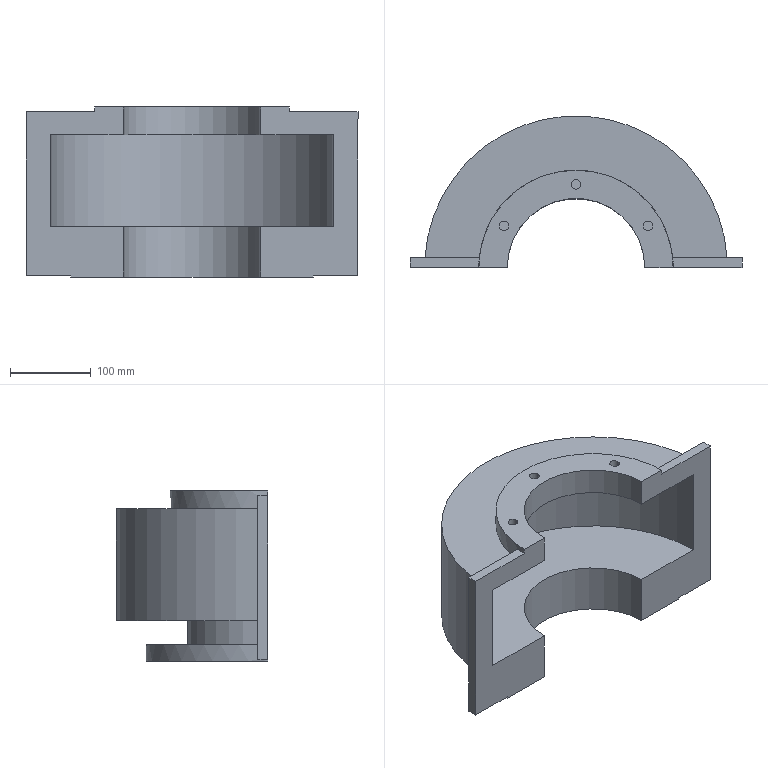Part | SolidWorks | features ICE 6, HoleWzd 2, Extrusion 1, RevCut 1 | 1 solid | 34 faces | box 410 x 187 x 210 mm | volume 2846531 mm3 | cylinder 17 | plane 17 | commonest cylinder face diameters 12 x6 16 x4 170 x2 198 x1 240 x1 300 x1
STEP:
#1=CARTESIAN_POINT('',(515.231,337.244,-184.693));
#2=VERTEX_POINT('',#1);
#3=CARTESIAN_POINT('',(527.231,337.244,-184.693));
#4=VERTEX_POINT('',#3);
#5=CARTESIAN_POINT('',(521.231,337.244,-184.693));
#6=DIRECTION('',(0.,0.,1.));
#7=DIRECTION('',(1.,0.,0.));
#8=AXIS2_PLACEMENT_3D('',#5,#6,#7);
#9=CIRCLE('',#8,6.);
#10=EDGE_CURVE('',#2,#4,#9,.T.);
#11=ORIENTED_EDGE('',*,*,#10,.F.);
#12=CARTESIAN_POINT('',(515.231,337.244,-150.693));
#13=VERTEX_POINT('',#12);
#14=CARTESIAN_POINT('',(515.231,337.244,-150.693));
#15=DIRECTION('',(0.,0.,1.));
#16=VECTOR('',#15,1000.);
#17=LINE('',#14,#16);
#18=EDGE_CURVE('',#2,#13,#17,.T.);
#19=ORIENTED_EDGE('',*,*,#18,.T.);
#20=CARTESIAN_POINT('',(527.231,337.244,-150.693));
#21=VERTEX_POINT('',#20);
#22=CARTESIAN_POINT('',(521.231,337.244,-150.693));
#23=DIRECTION('',(0.,0.,1.));
#24=DIRECTION('',(1.,0.,0.));
#25=AXIS2_PLACEMENT_3D('',#22,#23,#24);
#26=CIRCLE('',#25,6.);
#27=EDGE_CURVE('',#13,#21,#26,.T.);
#28=ORIENTED_EDGE('',*,*,#27,.T.);
#29=CARTESIAN_POINT('',(527.231,337.244,-150.693));
#30=DIRECTION('',(0.,0.,1.));
#31=VECTOR('',#30,1000.);
#32=LINE('',#29,#31);
#33=EDGE_CURVE('',#4,#21,#32,.T.);
#34=ORIENTED_EDGE('',*,*,#33,.F.);
#35=EDGE_LOOP('',(#11,#19,#28,#34));
#36=FACE_OUTER_BOUND('',#35,.T.);
#37=CARTESIAN_POINT('',(521.231,337.244,-150.693));
#38=DIRECTION('',(0.,0.,1.));
#39=DIRECTION('',(1.,0.,0.));
#40=AXIS2_PLACEMENT_3D('',#37,#38,#39);
#41=CYLINDRICAL_SURFACE('',#40,6.);
#42=ADVANCED_FACE('',(#36),#41,.F.);
#43=CARTESIAN_POINT('',(426.463,285.994,-184.693));
#44=VERTEX_POINT('',#43);
#45=CARTESIAN_POINT('',(438.463,285.994,-184.693));
#46=VERTEX_POINT('',#45);
#47=CARTESIAN_POINT('',(432.463,285.994,-184.693));
#48=DIRECTION('',(0.,0.,1.));
#49=DIRECTION('',(1.,0.,0.));
#50=AXIS2_PLACEMENT_3D('',#47,#48,#49);
#51=CIRCLE('',#50,6.);
#52=EDGE_CURVE('',#44,#46,#51,.T.);
#53=ORIENTED_EDGE('',*,*,#52,.F.);
#54=CARTESIAN_POINT('',(426.463,285.994,-150.693));
#55=VERTEX_POINT('',#54);
#56=CARTESIAN_POINT('',(426.463,285.994,-150.693));
#57=DIRECTION('',(0.,0.,1.));
#58=VECTOR('',#57,1000.);
#59=LINE('',#56,#58);
#60=EDGE_CURVE('',#44,#55,#59,.T.);
#61=ORIENTED_EDGE('',*,*,#60,.T.);
#62=CARTESIAN_POINT('',(438.463,285.994,-150.693));
#63=VERTEX_POINT('',#62);
#64=CARTESIAN_POINT('',(432.463,285.994,-150.693));
#65=DIRECTION('',(0.,0.,1.));
#66=DIRECTION('',(1.,0.,0.));
#67=AXIS2_PLACEMENT_3D('',#64,#65,#66);
#68=CIRCLE('',#67,6.);
#69=EDGE_CURVE('',#55,#63,#68,.T.);
#70=ORIENTED_EDGE('',*,*,#69,.T.);
#71=CARTESIAN_POINT('',(438.463,285.994,-150.693));
#72=DIRECTION('',(0.,0.,1.));
#73=VECTOR('',#72,1000.);
#74=LINE('',#71,#73);
#75=EDGE_CURVE('',#46,#63,#74,.T.);
#76=ORIENTED_EDGE('',*,*,#75,.F.);
#77=EDGE_LOOP('',(#53,#61,#70,#76));
#78=FACE_OUTER_BOUND('',#77,.T.);
#79=CARTESIAN_POINT('',(432.463,285.994,-150.693));
#80=DIRECTION('',(0.,0.,1.));
#81=DIRECTION('',(1.,0.,0.));
#82=AXIS2_PLACEMENT_3D('',#79,#80,#81);
#83=CYLINDRICAL_SURFACE('',#82,6.);
#84=ADVANCED_FACE('',(#78),#83,.F.);
#85=CARTESIAN_POINT('',(603.998,285.994,-184.693));
#86=VERTEX_POINT('',#85);
#87=CARTESIAN_POINT('',(615.998,285.994,-184.693));
#88=VERTEX_POINT('',#87);
#89=CARTESIAN_POINT('',(609.998,285.994,-184.693));
#90=DIRECTION('',(0.,0.,1.));
#91=DIRECTION('',(1.,0.,0.));
#92=AXIS2_PLACEMENT_3D('',#89,#90,#91);
#93=CIRCLE('',#92,6.);
#94=EDGE_CURVE('',#86,#88,#93,.T.);
#95=ORIENTED_EDGE('',*,*,#94,.F.);
#96=CARTESIAN_POINT('',(603.998,285.994,-150.693));
#97=VERTEX_POINT('',#96);
#98=CARTESIAN_POINT('',(603.998,285.994,-150.693));
#99=DIRECTION('',(0.,0.,1.));
#100=VECTOR('',#99,1000.);
#101=LINE('',#98,#100);
#102=EDGE_CURVE('',#86,#97,#101,.T.);
#103=ORIENTED_EDGE('',*,*,#102,.T.);
#104=CARTESIAN_POINT('',(615.998,285.994,-150.693));
#105=VERTEX_POINT('',#104);
#106=CARTESIAN_POINT('',(609.998,285.994,-150.693));
#107=DIRECTION('',(0.,0.,1.));
#108=DIRECTION('',(1.,0.,0.));
#109=AXIS2_PLACEMENT_3D('',#106,#107,#108);
#110=CIRCLE('',#109,6.);
#111=EDGE_CURVE('',#97,#105,#110,.T.);
#112=ORIENTED_EDGE('',*,*,#111,.T.);
#113=CARTESIAN_POINT('',(615.998,285.994,-150.693));
#114=DIRECTION('',(0.,0.,1.));
#115=VECTOR('',#114,1000.);
#116=LINE('',#113,#115);
#117=EDGE_CURVE('',#88,#105,#116,.T.);
#118=ORIENTED_EDGE('',*,*,#117,.F.);
#119=EDGE_LOOP('',(#95,#103,#112,#118));
#120=FACE_OUTER_BOUND('',#119,.T.);
#121=CARTESIAN_POINT('',(609.998,285.994,-150.693));
#122=DIRECTION('',(0.,0.,1.));
#123=DIRECTION('',(1.,0.,0.));
#124=AXIS2_PLACEMENT_3D('',#121,#122,#123);
#125=CYLINDRICAL_SURFACE('',#124,6.);
#126=ADVANCED_FACE('',(#120),#125,.F.);
#127=CARTESIAN_POINT('',(413.638,292.244,-360.693));
#128=VERTEX_POINT('',#127);
#129=CARTESIAN_POINT('',(429.638,292.244,-360.693));
#130=VERTEX_POINT('',#129);
#131=CARTESIAN_POINT('',(421.638,292.244,-360.693));
#132=DIRECTION('',(0.,0.,1.));
#133=DIRECTION('',(1.,0.,0.));
#134=AXIS2_PLACEMENT_3D('',#131,#132,#133);
#135=CIRCLE('',#134,8.);
#136=EDGE_CURVE('',#128,#130,#135,.T.);
#137=ORIENTED_EDGE('',*,*,#136,.F.);
#138=CARTESIAN_POINT('',(413.638,292.244,-340.693));
#139=VERTEX_POINT('',#138);
#140=CARTESIAN_POINT('',(413.638,292.244,-340.693));
#141=DIRECTION('',(0.,0.,1.));
#142=VECTOR('',#141,1000.);
#143=LINE('',#140,#142);
#144=EDGE_CURVE('',#128,#139,#143,.T.);
#145=ORIENTED_EDGE('',*,*,#144,.T.);
#146=CARTESIAN_POINT('',(429.638,292.244,-340.693));
#147=VERTEX_POINT('',#146);
#148=CARTESIAN_POINT('',(421.638,292.244,-340.693));
#149=DIRECTION('',(0.,0.,1.));
#150=DIRECTION('',(1.,0.,0.));
#151=AXIS2_PLACEMENT_3D('',#148,#149,#150);
#152=CIRCLE('',#151,8.);
#153=EDGE_CURVE('',#139,#147,#152,.T.);
#154=ORIENTED_EDGE('',*,*,#153,.T.);
#155=CARTESIAN_POINT('',(429.638,292.244,-340.693));
#156=DIRECTION('',(0.,0.,1.));
#157=VECTOR('',#156,1000.);
#158=LINE('',#155,#157);
#159=EDGE_CURVE('',#130,#147,#158,.T.);
#160=ORIENTED_EDGE('',*,*,#159,.F.);
#161=EDGE_LOOP('',(#137,#145,#154,#160));
#162=FACE_OUTER_BOUND('',#161,.T.);
#163=CARTESIAN_POINT('',(421.638,292.244,-340.693));
#164=DIRECTION('',(0.,0.,1.));
#165=DIRECTION('',(1.,0.,0.));
#166=AXIS2_PLACEMENT_3D('',#163,#164,#165);
#167=CYLINDRICAL_SURFACE('',#166,8.);
#168=ADVANCED_FACE('',(#162),#167,.F.);
#169=CARTESIAN_POINT('',(612.824,292.244,-360.693));
#170=VERTEX_POINT('',#169);
#171=CARTESIAN_POINT('',(628.824,292.244,-360.693));
#172=VERTEX_POINT('',#171);
#173=CARTESIAN_POINT('',(620.824,292.244,-360.693));
#174=DIRECTION('',(0.,0.,1.));
#175=DIRECTION('',(1.,0.,0.));
#176=AXIS2_PLACEMENT_3D('',#173,#174,#175);
#177=CIRCLE('',#176,8.);
#178=EDGE_CURVE('',#170,#172,#177,.T.);
#179=ORIENTED_EDGE('',*,*,#178,.F.);
#180=CARTESIAN_POINT('',(612.824,292.244,-340.693));
#181=VERTEX_POINT('',#180);
#182=CARTESIAN_POINT('',(612.824,292.244,-340.693));
#183=DIRECTION('',(0.,0.,1.));
#184=VECTOR('',#183,1000.);
#185=LINE('',#182,#184);
#186=EDGE_CURVE('',#170,#181,#185,.T.);
#187=ORIENTED_EDGE('',*,*,#186,.T.);
#188=CARTESIAN_POINT('',(628.824,292.244,-340.693));
#189=VERTEX_POINT('',#188);
#190=CARTESIAN_POINT('',(620.824,292.244,-340.693));
#191=DIRECTION('',(0.,0.,1.));
#192=DIRECTION('',(1.,0.,0.));
#193=AXIS2_PLACEMENT_3D('',#190,#191,#192);
#194=CIRCLE('',#193,8.);
#195=EDGE_CURVE('',#181,#189,#194,.T.);
#196=ORIENTED_EDGE('',*,*,#195,.T.);
#197=CARTESIAN_POINT('',(628.824,292.244,-340.693));
#198=DIRECTION('',(0.,0.,1.));
#199=VECTOR('',#198,1000.);
#200=LINE('',#197,#199);
#201=EDGE_CURVE('',#172,#189,#200,.T.);
#202=ORIENTED_EDGE('',*,*,#201,.F.);
#203=EDGE_LOOP('',(#179,#187,#196,#202));
#204=FACE_OUTER_BOUND('',#203,.T.);
#205=CARTESIAN_POINT('',(620.824,292.244,-340.693));
#206=DIRECTION('',(0.,0.,1.));
#207=DIRECTION('',(1.,0.,0.));
#208=AXIS2_PLACEMENT_3D('',#205,#206,#207);
#209=CYLINDRICAL_SURFACE('',#208,8.);
#210=ADVANCED_FACE('',(#204),#209,.F.);
#211=CARTESIAN_POINT('',(521.231,337.244,-150.693));
#212=DIRECTION('',(0.,0.,1.));
#213=DIRECTION('',(1.,0.,0.));
#214=AXIS2_PLACEMENT_3D('',#211,#212,#213);
#215=CIRCLE('',#214,6.);
#216=EDGE_CURVE('',#21,#13,#215,.T.);
#217=ORIENTED_EDGE('',*,*,#216,.F.);
#218=ORIENTED_EDGE('',*,*,#27,.F.);
#219=EDGE_LOOP('',(#217,#218));
#220=FACE_BOUND('',#219,.T.);
#221=CARTESIAN_POINT('',(401.231,234.744,-150.693));
#222=VERTEX_POINT('',#221);
#223=CARTESIAN_POINT('',(436.231,234.744,-150.693));
#224=VERTEX_POINT('',#223);
#225=CARTESIAN_POINT('',(641.231,234.744,-150.693));
#226=DIRECTION('',(1.,0.,0.));
#227=VECTOR('',#226,1000.);
#228=LINE('',#225,#227);
#229=EDGE_CURVE('',#222,#224,#228,.T.);
#230=ORIENTED_EDGE('',*,*,#229,.T.);
#231=CARTESIAN_POINT('',(606.231,234.744,-150.693));
#232=VERTEX_POINT('',#231);
#233=CARTESIAN_POINT('',(521.231,234.744,-150.693));
#234=DIRECTION('',(0.,0.,1.));
#235=DIRECTION('',(1.,0.,0.));
#236=AXIS2_PLACEMENT_3D('',#233,#234,#235);
#237=CIRCLE('',#236,85.);
#238=EDGE_CURVE('',#232,#224,#237,.T.);
#239=ORIENTED_EDGE('',*,*,#238,.F.);
#240=CARTESIAN_POINT('',(641.231,234.744,-150.693));
#241=VERTEX_POINT('',#240);
#242=CARTESIAN_POINT('',(641.231,234.744,-150.693));
#243=DIRECTION('',(1.,0.,0.));
#244=VECTOR('',#243,1000.);
#245=LINE('',#242,#244);
#246=EDGE_CURVE('',#232,#241,#245,.T.);
#247=ORIENTED_EDGE('',*,*,#246,.T.);
#248=CARTESIAN_POINT('',(521.231,234.744,-150.693));
#249=DIRECTION('',(0.,0.,1.));
#250=DIRECTION('',(-1.,0.,0.));
#251=AXIS2_PLACEMENT_3D('',#248,#249,#250);
#252=CIRCLE('',#251,120.);
#253=EDGE_CURVE('',#241,#222,#252,.T.);
#254=ORIENTED_EDGE('',*,*,#253,.T.);
#255=EDGE_LOOP('',(#230,#239,#247,#254));
#256=FACE_OUTER_BOUND('',#255,.T.);
#257=CARTESIAN_POINT('',(609.998,285.994,-150.693));
#258=DIRECTION('',(0.,0.,1.));
#259=DIRECTION('',(1.,0.,0.));
#260=AXIS2_PLACEMENT_3D('',#257,#258,#259);
#261=CIRCLE('',#260,6.);
#262=EDGE_CURVE('',#105,#97,#261,.T.);
#263=ORIENTED_EDGE('',*,*,#262,.F.);
#264=ORIENTED_EDGE('',*,*,#111,.F.);
#265=EDGE_LOOP('',(#263,#264));
#266=FACE_BOUND('',#265,.T.);
#267=CARTESIAN_POINT('',(432.463,285.994,-150.693));
#268=DIRECTION('',(0.,0.,1.));
#269=DIRECTION('',(1.,0.,0.));
#270=AXIS2_PLACEMENT_3D('',#267,#268,#269);
#271=CIRCLE('',#270,6.);
#272=EDGE_CURVE('',#63,#55,#271,.T.);
#273=ORIENTED_EDGE('',*,*,#272,.F.);
#274=ORIENTED_EDGE('',*,*,#69,.F.);
#275=EDGE_LOOP('',(#273,#274));
#276=FACE_BOUND('',#275,.T.);
#277=CARTESIAN_POINT('',(521.231,234.744,-150.693));
#278=DIRECTION('',(0.,0.,-1.));
#279=DIRECTION('',(-1.,0.,0.));
#280=AXIS2_PLACEMENT_3D('',#277,#278,#279);
#281=PLANE('',#280);
#282=ADVANCED_FACE('',(#220,#256,#266,#276),#281,.F.);
#283=CARTESIAN_POINT('',(436.231,234.744,-298.693));
#284=VERTEX_POINT('',#283);
#285=CARTESIAN_POINT('',(436.231,234.744,-360.693));
#286=VERTEX_POINT('',#285);
#287=CARTESIAN_POINT('',(436.231,234.744,-360.693));
#288=DIRECTION('',(0.,0.,-1.));
#289=VECTOR('',#288,1000.);
#290=LINE('',#287,#289);
#291=EDGE_CURVE('',#284,#286,#290,.T.);
#292=ORIENTED_EDGE('',*,*,#291,.F.);
#293=CARTESIAN_POINT('',(346.231,234.744,-298.693));
#294=VERTEX_POINT('',#293);
#295=CARTESIAN_POINT('',(726.231,234.744,-298.693));
#296=DIRECTION('',(1.,0.,0.));
#297=VECTOR('',#296,1000.);
#298=LINE('',#295,#297);
#299=EDGE_CURVE('',#294,#284,#298,.T.);
#300=ORIENTED_EDGE('',*,*,#299,.F.);
#301=CARTESIAN_POINT('',(346.231,234.744,-184.693));
#302=VERTEX_POINT('',#301);
#303=CARTESIAN_POINT('',(346.231,234.744,-360.693));
#304=DIRECTION('',(0.,0.,-1.));
#305=VECTOR('',#304,1000.);
#306=LINE('',#303,#305);
#307=EDGE_CURVE('',#302,#294,#306,.T.);
#308=ORIENTED_EDGE('',*,*,#307,.F.);
#309=CARTESIAN_POINT('',(436.231,234.744,-184.693));
#310=VERTEX_POINT('',#309);
#311=CARTESIAN_POINT('',(726.231,234.744,-184.693));
#312=DIRECTION('',(-1.,0.,0.));
#313=VECTOR('',#312,1000.);
#314=LINE('',#311,#313);
#315=EDGE_CURVE('',#310,#302,#314,.T.);
#316=ORIENTED_EDGE('',*,*,#315,.F.);
#317=CARTESIAN_POINT('',(436.231,234.744,-360.693));
#318=DIRECTION('',(0.,0.,-1.));
#319=VECTOR('',#318,1000.);
#320=LINE('',#317,#319);
#321=EDGE_CURVE('',#224,#310,#320,.T.);
#322=ORIENTED_EDGE('',*,*,#321,.F.);
#323=ORIENTED_EDGE('',*,*,#229,.F.);
#324=CARTESIAN_POINT('',(401.231,234.744,-156.693));
#325=VERTEX_POINT('',#324);
#326=CARTESIAN_POINT('',(401.231,234.744,-150.693));
#327=DIRECTION('',(0.,0.,-1.));
#328=VECTOR('',#327,1000.);
#329=LINE('',#326,#328);
#330=EDGE_CURVE('',#222,#325,#329,.T.);
#331=ORIENTED_EDGE('',*,*,#330,.T.);
#332=CARTESIAN_POINT('',(316.231,234.744,-156.693));
#333=VERTEX_POINT('',#332);
#334=CARTESIAN_POINT('',(726.231,234.744,-156.693));
#335=DIRECTION('',(-1.,0.,0.));
#336=VECTOR('',#335,1000.);
#337=LINE('',#334,#336);
#338=EDGE_CURVE('',#325,#333,#337,.T.);
#339=ORIENTED_EDGE('',*,*,#338,.T.);
#340=CARTESIAN_POINT('',(316.231,234.744,-358.693));
#341=VERTEX_POINT('',#340);
#342=CARTESIAN_POINT('',(316.231,234.744,-156.693));
#343=DIRECTION('',(0.,0.,-1.));
#344=VECTOR('',#343,1000.);
#345=LINE('',#342,#344);
#346=EDGE_CURVE('',#333,#341,#345,.T.);
#347=ORIENTED_EDGE('',*,*,#346,.T.);
#348=CARTESIAN_POINT('',(371.231,234.744,-358.693));
#349=VERTEX_POINT('',#348);
#350=CARTESIAN_POINT('',(726.231,234.744,-358.693));
#351=DIRECTION('',(-1.,0.,0.));
#352=VECTOR('',#351,1000.);
#353=LINE('',#350,#352);
#354=EDGE_CURVE('',#349,#341,#353,.T.);
#355=ORIENTED_EDGE('',*,*,#354,.F.);
#356=CARTESIAN_POINT('',(371.231,234.744,-360.693));
#357=VERTEX_POINT('',#356);
#358=CARTESIAN_POINT('',(371.231,234.744,-360.693));
#359=DIRECTION('',(0.,0.,1.));
#360=VECTOR('',#359,1000.);
#361=LINE('',#358,#360);
#362=EDGE_CURVE('',#357,#349,#361,.T.);
#363=ORIENTED_EDGE('',*,*,#362,.F.);
#364=CARTESIAN_POINT('',(371.231,234.744,-360.693));
#365=DIRECTION('',(-1.,0.,0.));
#366=VECTOR('',#365,1000.);
#367=LINE('',#364,#366);
#368=EDGE_CURVE('',#286,#357,#367,.T.);
#369=ORIENTED_EDGE('',*,*,#368,.F.);
#370=EDGE_LOOP('',(#292,#300,#308,#316,#322,#323,#331,#339,#347,#355,#363,#369));
#371=FACE_OUTER_BOUND('',#370,.T.);
#372=CARTESIAN_POINT('',(726.231,234.744,-156.693));
#373=DIRECTION('',(0.,-1.,0.));
#374=DIRECTION('',(1.,0.,0.));
#375=AXIS2_PLACEMENT_3D('',#372,#373,#374);
#376=PLANE('',#375);
#377=ADVANCED_FACE('',(#371),#376,.T.);
#378=CARTESIAN_POINT('',(670.75,246.744,-340.693));
#379=VERTEX_POINT('',#378);
#380=CARTESIAN_POINT('',(619.501,246.744,-340.693));
#381=VERTEX_POINT('',#380);
#382=CARTESIAN_POINT('',(707.845,246.744,-340.693));
#383=DIRECTION('',(-1.,0.,0.));
#384=VECTOR('',#383,1000.);
#385=LINE('',#382,#384);
#386=EDGE_CURVE('',#379,#381,#385,.T.);
#387=ORIENTED_EDGE('',*,*,#386,.T.);
#388=CARTESIAN_POINT('',(619.501,246.744,-310.693));
#389=VERTEX_POINT('',#388);
#390=CARTESIAN_POINT('',(619.501,246.744,-310.693));
#391=DIRECTION('',(0.,0.,-1.));
#392=VECTOR('',#391,1000.);
#393=LINE('',#390,#392);
#394=EDGE_CURVE('',#389,#381,#393,.T.);
#395=ORIENTED_EDGE('',*,*,#394,.F.);
#396=CARTESIAN_POINT('',(707.845,246.744,-310.693));
#397=VERTEX_POINT('',#396);
#398=CARTESIAN_POINT('',(707.845,246.744,-310.693));
#399=DIRECTION('',(-1.,0.,0.));
#400=VECTOR('',#399,1000.);
#401=LINE('',#398,#400);
#402=EDGE_CURVE('',#397,#389,#401,.T.);
#403=ORIENTED_EDGE('',*,*,#402,.F.);
#404=CARTESIAN_POINT('',(707.845,246.744,-172.693));
#405=VERTEX_POINT('',#404);
#406=CARTESIAN_POINT('',(707.845,246.744,-156.693));
#407=DIRECTION('',(0.,0.,-1.));
#408=VECTOR('',#407,1000.);
#409=LINE('',#406,#408);
#410=EDGE_CURVE('',#405,#397,#409,.T.);
#411=ORIENTED_EDGE('',*,*,#410,.F.);
#412=CARTESIAN_POINT('',(640.629,246.744,-172.693));
#413=VERTEX_POINT('',#412);
#414=CARTESIAN_POINT('',(640.629,246.744,-172.693));
#415=DIRECTION('',(1.,0.,0.));
#416=VECTOR('',#415,1000.);
#417=LINE('',#414,#416);
#418=EDGE_CURVE('',#413,#405,#417,.T.);
#419=ORIENTED_EDGE('',*,*,#418,.F.);
#420=CARTESIAN_POINT('',(640.629,246.744,-156.693));
#421=VERTEX_POINT('',#420);
#422=CARTESIAN_POINT('',(640.629,246.744,-172.693));
#423=DIRECTION('',(0.,0.,1.));
#424=VECTOR('',#423,1000.);
#425=LINE('',#422,#424);
#426=EDGE_CURVE('',#413,#421,#425,.T.);
#427=ORIENTED_EDGE('',*,*,#426,.T.);
#428=CARTESIAN_POINT('',(726.231,246.744,-156.693));
#429=VERTEX_POINT('',#428);
#430=CARTESIAN_POINT('',(707.845,246.744,-156.693));
#431=DIRECTION('',(1.,0.,0.));
#432=VECTOR('',#431,1000.);
#433=LINE('',#430,#432);
#434=EDGE_CURVE('',#421,#429,#433,.T.);
#435=ORIENTED_EDGE('',*,*,#434,.T.);
#436=CARTESIAN_POINT('',(726.231,246.744,-358.693));
#437=VERTEX_POINT('',#436);
#438=CARTESIAN_POINT('',(726.231,246.744,-156.693));
#439=DIRECTION('',(0.,0.,-1.));
#440=VECTOR('',#439,1000.);
#441=LINE('',#438,#440);
#442=EDGE_CURVE('',#429,#437,#441,.T.);
#443=ORIENTED_EDGE('',*,*,#442,.T.);
#444=CARTESIAN_POINT('',(670.75,246.744,-358.693));
#445=VERTEX_POINT('',#444);
#446=CARTESIAN_POINT('',(707.845,246.744,-358.693));
#447=DIRECTION('',(1.,0.,0.));
#448=VECTOR('',#447,1000.);
#449=LINE('',#446,#448);
#450=EDGE_CURVE('',#445,#437,#449,.T.);
#451=ORIENTED_EDGE('',*,*,#450,.F.);
#452=CARTESIAN_POINT('',(670.75,246.744,-340.693));
#453=DIRECTION('',(0.,0.,-1.));
#454=VECTOR('',#453,1000.);
#455=LINE('',#452,#454);
#456=EDGE_CURVE('',#379,#445,#455,.T.);
#457=ORIENTED_EDGE('',*,*,#456,.F.);
#458=EDGE_LOOP('',(#387,#395,#403,#411,#419,#427,#435,#443,#451,#457));
#459=FACE_OUTER_BOUND('',#458,.T.);
#460=CARTESIAN_POINT('',(316.231,246.744,-156.693));
#461=DIRECTION('',(0.,1.,0.));
#462=DIRECTION('',(0.,0.,1.));
#463=AXIS2_PLACEMENT_3D('',#460,#461,#462);
#464=PLANE('',#463);
#465=ADVANCED_FACE('',(#459),#464,.T.);
#466=CARTESIAN_POINT('',(422.961,246.744,-310.693));
#467=VERTEX_POINT('',#466);
#468=CARTESIAN_POINT('',(334.616,246.744,-310.693));
#469=VERTEX_POINT('',#468);
#470=CARTESIAN_POINT('',(707.845,246.744,-310.693));
#471=DIRECTION('',(-1.,0.,0.));
#472=VECTOR('',#471,1000.);
#473=LINE('',#470,#472);
#474=EDGE_CURVE('',#467,#469,#473,.T.);
#475=ORIENTED_EDGE('',*,*,#474,.F.);
#476=CARTESIAN_POINT('',(422.961,246.744,-340.693));
#477=VERTEX_POINT('',#476);
#478=CARTESIAN_POINT('',(422.961,246.744,-310.693));
#479=DIRECTION('',(0.,0.,-1.));
#480=VECTOR('',#479,1000.);
#481=LINE('',#478,#480);
#482=EDGE_CURVE('',#467,#477,#481,.T.);
#483=ORIENTED_EDGE('',*,*,#482,.T.);
#484=CARTESIAN_POINT('',(371.711,246.744,-340.693));
#485=VERTEX_POINT('',#484);
#486=CARTESIAN_POINT('',(707.845,246.744,-340.693));
#487=DIRECTION('',(-1.,0.,0.));
#488=VECTOR('',#487,1000.);
#489=LINE('',#486,#488);
#490=EDGE_CURVE('',#477,#485,#489,.T.);
#491=ORIENTED_EDGE('',*,*,#490,.T.);
#492=CARTESIAN_POINT('',(371.711,246.744,-358.693));
#493=VERTEX_POINT('',#492);
#494=CARTESIAN_POINT('',(371.711,246.744,-340.693));
#495=DIRECTION('',(0.,0.,-1.));
#496=VECTOR('',#495,1000.);
#497=LINE('',#494,#496);
#498=EDGE_CURVE('',#485,#493,#497,.T.);
#499=ORIENTED_EDGE('',*,*,#498,.T.);
#500=CARTESIAN_POINT('',(316.231,246.744,-358.693));
#501=VERTEX_POINT('',#500);
#502=CARTESIAN_POINT('',(316.231,246.744,-358.693));
#503=DIRECTION('',(1.,0.,0.));
#504=VECTOR('',#503,1000.);
#505=LINE('',#502,#504);
#506=EDGE_CURVE('',#501,#493,#505,.T.);
#507=ORIENTED_EDGE('',*,*,#506,.F.);
#508=CARTESIAN_POINT('',(316.231,246.744,-156.693));
#509=VERTEX_POINT('',#508);
#510=CARTESIAN_POINT('',(316.231,246.744,-156.693));
#511=DIRECTION('',(0.,0.,-1.));
#512=VECTOR('',#511,1000.);
#513=LINE('',#510,#512);
#514=EDGE_CURVE('',#509,#501,#513,.T.);
#515=ORIENTED_EDGE('',*,*,#514,.F.);
#516=CARTESIAN_POINT('',(401.832,246.744,-156.693));
#517=VERTEX_POINT('',#516);
#518=CARTESIAN_POINT('',(316.231,246.744,-156.693));
#519=DIRECTION('',(1.,0.,0.));
#520=VECTOR('',#519,1000.);
#521=LINE('',#518,#520);
#522=EDGE_CURVE('',#509,#517,#521,.T.);
#523=ORIENTED_EDGE('',*,*,#522,.T.);
#524=CARTESIAN_POINT('',(401.832,246.744,-172.693));
#525=VERTEX_POINT('',#524);
#526=CARTESIAN_POINT('',(401.832,246.744,-172.693));
#527=DIRECTION('',(0.,0.,1.));
#528=VECTOR('',#527,1000.);
#529=LINE('',#526,#528);
#530=EDGE_CURVE('',#525,#517,#529,.T.);
#531=ORIENTED_EDGE('',*,*,#530,.F.);
#532=CARTESIAN_POINT('',(334.616,246.744,-172.693));
#533=VERTEX_POINT('',#532);
#534=CARTESIAN_POINT('',(334.616,246.744,-172.693));
#535=DIRECTION('',(1.,0.,0.));
#536=VECTOR('',#535,1000.);
#537=LINE('',#534,#536);
#538=EDGE_CURVE('',#533,#525,#537,.T.);
#539=ORIENTED_EDGE('',*,*,#538,.F.);
#540=CARTESIAN_POINT('',(334.616,246.744,-156.693));
#541=DIRECTION('',(0.,0.,-1.));
#542=VECTOR('',#541,1000.);
#543=LINE('',#540,#542);
#544=EDGE_CURVE('',#533,#469,#543,.T.);
#545=ORIENTED_EDGE('',*,*,#544,.T.);
#546=EDGE_LOOP('',(#475,#483,#491,#499,#507,#515,#523,#531,#539,#545));
#547=FACE_OUTER_BOUND('',#546,.T.);
#548=CARTESIAN_POINT('',(316.231,246.744,-156.693));
#549=DIRECTION('',(0.,1.,0.));
#550=DIRECTION('',(0.,0.,1.));
#551=AXIS2_PLACEMENT_3D('',#548,#549,#550);
#552=PLANE('',#551);
#553=ADVANCED_FACE('',(#547),#552,.T.);
#554=CARTESIAN_POINT('',(421.638,292.244,-340.693));
#555=DIRECTION('',(0.,0.,1.));
#556=DIRECTION('',(1.,0.,0.));
#557=AXIS2_PLACEMENT_3D('',#554,#555,#556);
#558=CIRCLE('',#557,8.);
#559=EDGE_CURVE('',#147,#139,#558,.T.);
#560=ORIENTED_EDGE('',*,*,#559,.F.);
#561=ORIENTED_EDGE('',*,*,#153,.F.);
#562=EDGE_LOOP('',(#560,#561));
#563=FACE_BOUND('',#562,.T.);
#564=CARTESIAN_POINT('',(620.824,292.244,-340.693));
#565=DIRECTION('',(0.,0.,1.));
#566=DIRECTION('',(1.,0.,0.));
#567=AXIS2_PLACEMENT_3D('',#564,#565,#566);
#568=CIRCLE('',#567,8.);
#569=EDGE_CURVE('',#189,#181,#568,.T.);
#570=ORIENTED_EDGE('',*,*,#569,.F.);
#571=ORIENTED_EDGE('',*,*,#195,.F.);
#572=EDGE_LOOP('',(#570,#571));
#573=FACE_BOUND('',#572,.T.);
#574=CARTESIAN_POINT('',(521.231,234.744,-340.693));
#575=DIRECTION('',(0.,0.,1.));
#576=DIRECTION('',(-1.,0.,0.));
#577=AXIS2_PLACEMENT_3D('',#574,#575,#576);
#578=CIRCLE('',#577,99.);
#579=EDGE_CURVE('',#381,#477,#578,.T.);
#580=ORIENTED_EDGE('',*,*,#579,.F.);
#581=ORIENTED_EDGE('',*,*,#386,.F.);
#582=CARTESIAN_POINT('',(521.231,234.744,-340.693));
#583=DIRECTION('',(0.,0.,1.));
#584=DIRECTION('',(1.,0.,0.));
#585=AXIS2_PLACEMENT_3D('',#582,#583,#584);
#586=CIRCLE('',#585,150.);
#587=EDGE_CURVE('',#379,#485,#586,.T.);
#588=ORIENTED_EDGE('',*,*,#587,.T.);
#589=ORIENTED_EDGE('',*,*,#490,.F.);
#590=EDGE_LOOP('',(#580,#581,#588,#589));
#591=FACE_OUTER_BOUND('',#590,.T.);
#592=CARTESIAN_POINT('',(521.231,234.744,-340.693));
#593=DIRECTION('',(0.,0.,-1.));
#594=DIRECTION('',(-1.,0.,0.));
#595=AXIS2_PLACEMENT_3D('',#592,#593,#594);
#596=PLANE('',#595);
#597=ADVANCED_FACE('',(#563,#573,#591),#596,.F.);
#598=ORIENTED_EDGE('',*,*,#402,.T.);
#599=CARTESIAN_POINT('',(521.231,234.744,-310.693));
#600=DIRECTION('',(0.,0.,1.));
#601=DIRECTION('',(-1.,0.,0.));
#602=AXIS2_PLACEMENT_3D('',#599,#600,#601);
#603=CIRCLE('',#602,99.);
#604=EDGE_CURVE('',#389,#467,#603,.T.);
#605=ORIENTED_EDGE('',*,*,#604,.T.);
#606=ORIENTED_EDGE('',*,*,#474,.T.);
#607=CARTESIAN_POINT('',(521.231,234.744,-310.693));
#608=DIRECTION('',(0.,0.,-1.));
#609=DIRECTION('',(-1.,0.,0.));
#610=AXIS2_PLACEMENT_3D('',#607,#608,#609);
#611=CIRCLE('',#610,187.);
#612=EDGE_CURVE('',#469,#397,#611,.T.);
#613=ORIENTED_EDGE('',*,*,#612,.T.);
#614=EDGE_LOOP('',(#598,#605,#606,#613));
#615=FACE_OUTER_BOUND('',#614,.T.);
#616=CARTESIAN_POINT('',(521.231,234.744,-310.693));
#617=DIRECTION('',(0.,0.,-1.));
#618=DIRECTION('',(-1.,0.,0.));
#619=AXIS2_PLACEMENT_3D('',#616,#617,#618);
#620=PLANE('',#619);
#621=ADVANCED_FACE('',(#615),#620,.T.);
#622=CARTESIAN_POINT('',(641.231,234.744,-156.693));
#623=VERTEX_POINT('',#622);
#624=CARTESIAN_POINT('',(521.231,234.744,-156.693));
#625=DIRECTION('',(0.,0.,1.));
#626=DIRECTION('',(-1.,0.,0.));
#627=AXIS2_PLACEMENT_3D('',#624,#625,#626);
#628=CIRCLE('',#627,120.);
#629=EDGE_CURVE('',#623,#421,#628,.T.);
#630=ORIENTED_EDGE('',*,*,#629,.F.);
#631=CARTESIAN_POINT('',(726.231,234.744,-156.693));
#632=VERTEX_POINT('',#631);
#633=CARTESIAN_POINT('',(726.231,234.744,-156.693));
#634=DIRECTION('',(-1.,0.,0.));
#635=VECTOR('',#634,1000.);
#636=LINE('',#633,#635);
#637=EDGE_CURVE('',#632,#623,#636,.T.);
#638=ORIENTED_EDGE('',*,*,#637,.F.);
#639=CARTESIAN_POINT('',(726.231,246.744,-156.693));
#640=DIRECTION('',(0.,-1.,0.));
#641=VECTOR('',#640,1000.);
#642=LINE('',#639,#641);
#643=EDGE_CURVE('',#429,#632,#642,.T.);
#644=ORIENTED_EDGE('',*,*,#643,.F.);
#645=ORIENTED_EDGE('',*,*,#434,.F.);
#646=EDGE_LOOP('',(#630,#638,#644,#645));
#647=FACE_OUTER_BOUND('',#646,.T.);
#648=CARTESIAN_POINT('',(521.231,234.744,-156.693));
#649=DIRECTION('',(0.,0.,-1.));
#650=DIRECTION('',(-1.,0.,0.));
#651=AXIS2_PLACEMENT_3D('',#648,#649,#650);
#652=PLANE('',#651);
#653=ADVANCED_FACE('',(#647),#652,.F.);
#654=CARTESIAN_POINT('',(521.231,234.744,-358.693));
#655=DIRECTION('',(0.,0.,-1.));
#656=DIRECTION('',(1.,0.,0.));
#657=AXIS2_PLACEMENT_3D('',#654,#655,#656);
#658=CIRCLE('',#657,150.);
#659=EDGE_CURVE('',#349,#493,#658,.T.);
#660=ORIENTED_EDGE('',*,*,#659,.F.);
#661=ORIENTED_EDGE('',*,*,#354,.T.);
#662=CARTESIAN_POINT('',(316.231,234.744,-358.693));
#663=DIRECTION('',(0.,1.,0.));
#664=VECTOR('',#663,1000.);
#665=LINE('',#662,#664);
#666=EDGE_CURVE('',#341,#501,#665,.T.);
#667=ORIENTED_EDGE('',*,*,#666,.T.);
#668=ORIENTED_EDGE('',*,*,#506,.T.);
#669=EDGE_LOOP('',(#660,#661,#667,#668));
#670=FACE_OUTER_BOUND('',#669,.T.);
#671=CARTESIAN_POINT('',(521.231,234.744,-358.693));
#672=DIRECTION('',(0.,0.,-1.));
#673=DIRECTION('',(-1.,0.,0.));
#674=AXIS2_PLACEMENT_3D('',#671,#672,#673);
#675=PLANE('',#674);
#676=ADVANCED_FACE('',(#670),#675,.T.);
#677=ORIENTED_EDGE('',*,*,#410,.T.);
#678=ORIENTED_EDGE('',*,*,#612,.F.);
#679=ORIENTED_EDGE('',*,*,#544,.F.);
#680=CARTESIAN_POINT('',(521.231,234.744,-172.693));
#681=DIRECTION('',(0.,0.,1.));
#682=DIRECTION('',(1.,0.,0.));
#683=AXIS2_PLACEMENT_3D('',#680,#681,#682);
#684=CIRCLE('',#683,187.);
#685=EDGE_CURVE('',#405,#533,#684,.T.);
#686=ORIENTED_EDGE('',*,*,#685,.F.);
#687=EDGE_LOOP('',(#677,#678,#679,#686));
#688=FACE_OUTER_BOUND('',#687,.T.);
#689=CARTESIAN_POINT('',(521.231,234.744,-156.693));
#690=DIRECTION('',(0.,0.,-1.));
#691=DIRECTION('',(-1.,0.,0.));
#692=AXIS2_PLACEMENT_3D('',#689,#690,#691);
#693=CYLINDRICAL_SURFACE('',#692,187.);
#694=ADVANCED_FACE('',(#688),#693,.T.);
#695=ORIENTED_EDGE('',*,*,#666,.F.);
#696=ORIENTED_EDGE('',*,*,#346,.F.);
#697=CARTESIAN_POINT('',(316.231,234.744,-156.693));
#698=DIRECTION('',(0.,1.,0.));
#699=VECTOR('',#698,1000.);
#700=LINE('',#697,#699);
#701=EDGE_CURVE('',#333,#509,#700,.T.);
#702=ORIENTED_EDGE('',*,*,#701,.T.);
#703=ORIENTED_EDGE('',*,*,#514,.T.);
#704=EDGE_LOOP('',(#695,#696,#702,#703));
#705=FACE_OUTER_BOUND('',#704,.T.);
#706=CARTESIAN_POINT('',(316.231,234.744,-156.693));
#707=DIRECTION('',(-1.,0.,0.));
#708=DIRECTION('',(0.,0.,1.));
#709=AXIS2_PLACEMENT_3D('',#706,#707,#708);
#710=PLANE('',#709);
#711=ADVANCED_FACE('',(#705),#710,.T.);
#712=CARTESIAN_POINT('',(606.231,234.744,-360.693));
#713=VERTEX_POINT('',#712);
#714=CARTESIAN_POINT('',(606.231,234.744,-298.693));
#715=VERTEX_POINT('',#714);
#716=CARTESIAN_POINT('',(606.231,234.744,-360.693));
#717=DIRECTION('',(0.,0.,1.));
#718=VECTOR('',#717,1000.);
#719=LINE('',#716,#718);
#720=EDGE_CURVE('',#713,#715,#719,.T.);
#721=ORIENTED_EDGE('',*,*,#720,.F.);
#722=CARTESIAN_POINT('',(671.231,234.744,-360.693));
#723=VERTEX_POINT('',#722);
#724=CARTESIAN_POINT('',(371.231,234.744,-360.693));
#725=DIRECTION('',(-1.,0.,0.));
#726=VECTOR('',#725,1000.);
#727=LINE('',#724,#726);
#728=EDGE_CURVE('',#723,#713,#727,.T.);
#729=ORIENTED_EDGE('',*,*,#728,.F.);
#730=CARTESIAN_POINT('',(671.231,234.744,-358.693));
#731=VERTEX_POINT('',#730);
#732=CARTESIAN_POINT('',(671.231,234.744,-360.693));
#733=DIRECTION('',(0.,0.,1.));
#734=VECTOR('',#733,1000.);
#735=LINE('',#732,#734);
#736=EDGE_CURVE('',#723,#731,#735,.T.);
#737=ORIENTED_EDGE('',*,*,#736,.T.);
#738=CARTESIAN_POINT('',(726.231,234.744,-358.693));
#739=VERTEX_POINT('',#738);
#740=CARTESIAN_POINT('',(726.231,234.744,-358.693));
#741=DIRECTION('',(-1.,0.,0.));
#742=VECTOR('',#741,1000.);
#743=LINE('',#740,#742);
#744=EDGE_CURVE('',#739,#731,#743,.T.);
#745=ORIENTED_EDGE('',*,*,#744,.F.);
#746=CARTESIAN_POINT('',(726.231,234.744,-156.693));
#747=DIRECTION('',(0.,0.,-1.));
#748=VECTOR('',#747,1000.);
#749=LINE('',#746,#748);
#750=EDGE_CURVE('',#632,#739,#749,.T.);
#751=ORIENTED_EDGE('',*,*,#750,.F.);
#752=ORIENTED_EDGE('',*,*,#637,.T.);
#753=CARTESIAN_POINT('',(641.231,234.744,-150.693));
#754=DIRECTION('',(0.,0.,-1.));
#755=VECTOR('',#754,1000.);
#756=LINE('',#753,#755);
#757=EDGE_CURVE('',#241,#623,#756,.T.);
#758=ORIENTED_EDGE('',*,*,#757,.F.);
#759=ORIENTED_EDGE('',*,*,#246,.F.);
#760=CARTESIAN_POINT('',(606.231,234.744,-184.693));
#761=VERTEX_POINT('',#760);
#762=CARTESIAN_POINT('',(606.231,234.744,-360.693));
#763=DIRECTION('',(0.,0.,1.));
#764=VECTOR('',#763,1000.);
#765=LINE('',#762,#764);
#766=EDGE_CURVE('',#761,#232,#765,.T.);
#767=ORIENTED_EDGE('',*,*,#766,.F.);
#768=CARTESIAN_POINT('',(696.231,234.744,-184.693));
#769=VERTEX_POINT('',#768);
#770=CARTESIAN_POINT('',(726.231,234.744,-184.693));
#771=DIRECTION('',(-1.,0.,0.));
#772=VECTOR('',#771,1000.);
#773=LINE('',#770,#772);
#774=EDGE_CURVE('',#769,#761,#773,.T.);
#775=ORIENTED_EDGE('',*,*,#774,.F.);
#776=CARTESIAN_POINT('',(696.231,234.744,-298.693));
#777=VERTEX_POINT('',#776);
#778=CARTESIAN_POINT('',(696.231,234.744,-360.693));
#779=DIRECTION('',(0.,0.,1.));
#780=VECTOR('',#779,1000.);
#781=LINE('',#778,#780);
#782=EDGE_CURVE('',#777,#769,#781,.T.);
#783=ORIENTED_EDGE('',*,*,#782,.F.);
#784=CARTESIAN_POINT('',(726.231,234.744,-298.693));
#785=DIRECTION('',(1.,0.,0.));
#786=VECTOR('',#785,1000.);
#787=LINE('',#784,#786);
#788=EDGE_CURVE('',#715,#777,#787,.T.);
#789=ORIENTED_EDGE('',*,*,#788,.F.);
#790=EDGE_LOOP('',(#721,#729,#737,#745,#751,#752,#758,#759,#767,#775,#783,#789));
#791=FACE_OUTER_BOUND('',#790,.T.);
#792=CARTESIAN_POINT('',(726.231,234.744,-156.693));
#793=DIRECTION('',(0.,-1.,0.));
#794=DIRECTION('',(1.,0.,0.));
#795=AXIS2_PLACEMENT_3D('',#792,#793,#794);
#796=PLANE('',#795);
#797=ADVANCED_FACE('',(#791),#796,.T.);
#798=CARTESIAN_POINT('',(726.231,246.744,-358.693));
#799=DIRECTION('',(0.,-1.,0.));
#800=VECTOR('',#799,1000.);
#801=LINE('',#798,#800);
#802=EDGE_CURVE('',#437,#739,#801,.T.);
#803=ORIENTED_EDGE('',*,*,#802,.F.);
#804=ORIENTED_EDGE('',*,*,#442,.F.);
#805=ORIENTED_EDGE('',*,*,#643,.T.);
#806=ORIENTED_EDGE('',*,*,#750,.T.);
#807=EDGE_LOOP('',(#803,#804,#805,#806));
#808=FACE_OUTER_BOUND('',#807,.T.);
#809=CARTESIAN_POINT('',(726.231,246.744,-156.693));
#810=DIRECTION('',(1.,0.,0.));
#811=DIRECTION('',(0.,0.,-1.));
#812=AXIS2_PLACEMENT_3D('',#809,#810,#811);
#813=PLANE('',#812);
#814=ADVANCED_FACE('',(#808),#813,.T.);
#815=CARTESIAN_POINT('',(521.231,234.744,-156.693));
#816=DIRECTION('',(0.,0.,1.));
#817=DIRECTION('',(-1.,0.,0.));
#818=AXIS2_PLACEMENT_3D('',#815,#816,#817);
#819=CIRCLE('',#818,120.);
#820=EDGE_CURVE('',#517,#325,#819,.T.);
#821=ORIENTED_EDGE('',*,*,#820,.F.);
#822=ORIENTED_EDGE('',*,*,#522,.F.);
#823=ORIENTED_EDGE('',*,*,#701,.F.);
#824=ORIENTED_EDGE('',*,*,#338,.F.);
#825=EDGE_LOOP('',(#821,#822,#823,#824));
#826=FACE_OUTER_BOUND('',#825,.T.);
#827=CARTESIAN_POINT('',(521.231,234.744,-156.693));
#828=DIRECTION('',(0.,0.,-1.));
#829=DIRECTION('',(-1.,0.,0.));
#830=AXIS2_PLACEMENT_3D('',#827,#828,#829);
#831=PLANE('',#830);
#832=ADVANCED_FACE('',(#826),#831,.F.);
#833=CARTESIAN_POINT('',(521.231,234.744,-358.693));
#834=DIRECTION('',(0.,0.,-1.));
#835=DIRECTION('',(1.,0.,0.));
#836=AXIS2_PLACEMENT_3D('',#833,#834,#835);
#837=CIRCLE('',#836,150.);
#838=EDGE_CURVE('',#445,#731,#837,.T.);
#839=ORIENTED_EDGE('',*,*,#838,.F.);
#840=ORIENTED_EDGE('',*,*,#450,.T.);
#841=ORIENTED_EDGE('',*,*,#802,.T.);
#842=ORIENTED_EDGE('',*,*,#744,.T.);
#843=EDGE_LOOP('',(#839,#840,#841,#842));
#844=FACE_OUTER_BOUND('',#843,.T.);
#845=CARTESIAN_POINT('',(521.231,234.744,-358.693));
#846=DIRECTION('',(0.,0.,-1.));
#847=DIRECTION('',(-1.,0.,0.));
#848=AXIS2_PLACEMENT_3D('',#845,#846,#847);
#849=PLANE('',#848);
#850=ADVANCED_FACE('',(#844),#849,.T.);
#851=ORIENTED_EDGE('',*,*,#530,.T.);
#852=ORIENTED_EDGE('',*,*,#820,.T.);
#853=ORIENTED_EDGE('',*,*,#330,.F.);
#854=ORIENTED_EDGE('',*,*,#253,.F.);
#855=ORIENTED_EDGE('',*,*,#757,.T.);
#856=ORIENTED_EDGE('',*,*,#629,.T.);
#857=ORIENTED_EDGE('',*,*,#426,.F.);
#858=CARTESIAN_POINT('',(521.231,234.744,-172.693));
#859=DIRECTION('',(0.,0.,-1.));
#860=DIRECTION('',(-1.,0.,0.));
#861=AXIS2_PLACEMENT_3D('',#858,#859,#860);
#862=CIRCLE('',#861,120.);
#863=EDGE_CURVE('',#525,#413,#862,.T.);
#864=ORIENTED_EDGE('',*,*,#863,.F.);
#865=EDGE_LOOP('',(#851,#852,#853,#854,#855,#856,#857,#864));
#866=FACE_OUTER_BOUND('',#865,.T.);
#867=CARTESIAN_POINT('',(521.231,234.744,-172.693));
#868=DIRECTION('',(0.,0.,1.));
#869=DIRECTION('',(1.,0.,0.));
#870=AXIS2_PLACEMENT_3D('',#867,#868,#869);
#871=CYLINDRICAL_SURFACE('',#870,120.);
#872=ADVANCED_FACE('',(#866),#871,.T.);
#873=ORIENTED_EDGE('',*,*,#863,.T.);
#874=ORIENTED_EDGE('',*,*,#418,.T.);
#875=ORIENTED_EDGE('',*,*,#685,.T.);
#876=ORIENTED_EDGE('',*,*,#538,.T.);
#877=EDGE_LOOP('',(#873,#874,#875,#876));
#878=FACE_OUTER_BOUND('',#877,.T.);
#879=CARTESIAN_POINT('',(521.231,234.744,-172.693));
#880=DIRECTION('',(0.,0.,-1.));
#881=DIRECTION('',(-1.,0.,0.));
#882=AXIS2_PLACEMENT_3D('',#879,#880,#881);
#883=PLANE('',#882);
#884=ADVANCED_FACE('',(#878),#883,.F.);
#885=ORIENTED_EDGE('',*,*,#456,.T.);
#886=ORIENTED_EDGE('',*,*,#838,.T.);
#887=ORIENTED_EDGE('',*,*,#736,.F.);
#888=CARTESIAN_POINT('',(521.231,234.744,-360.693));
#889=DIRECTION('',(0.,0.,-1.));
#890=DIRECTION('',(1.,0.,0.));
#891=AXIS2_PLACEMENT_3D('',#888,#889,#890);
#892=CIRCLE('',#891,150.);
#893=EDGE_CURVE('',#357,#723,#892,.T.);
#894=ORIENTED_EDGE('',*,*,#893,.F.);
#895=ORIENTED_EDGE('',*,*,#362,.T.);
#896=ORIENTED_EDGE('',*,*,#659,.T.);
#897=ORIENTED_EDGE('',*,*,#498,.F.);
#898=ORIENTED_EDGE('',*,*,#587,.F.);
#899=EDGE_LOOP('',(#885,#886,#887,#894,#895,#896,#897,#898));
#900=FACE_OUTER_BOUND('',#899,.T.);
#901=CARTESIAN_POINT('',(521.231,234.744,-340.693));
#902=DIRECTION('',(0.,0.,-1.));
#903=DIRECTION('',(-1.,0.,0.));
#904=AXIS2_PLACEMENT_3D('',#901,#902,#903);
#905=CYLINDRICAL_SURFACE('',#904,150.);
#906=ADVANCED_FACE('',(#900),#905,.T.);
#907=CARTESIAN_POINT('',(421.638,292.244,-360.693));
#908=DIRECTION('',(0.,0.,1.));
#909=DIRECTION('',(1.,0.,0.));
#910=AXIS2_PLACEMENT_3D('',#907,#908,#909);
#911=CIRCLE('',#910,8.);
#912=EDGE_CURVE('',#130,#128,#911,.T.);
#913=ORIENTED_EDGE('',*,*,#912,.T.);
#914=ORIENTED_EDGE('',*,*,#136,.T.);
#915=EDGE_LOOP('',(#913,#914));
#916=FACE_BOUND('',#915,.T.);
#917=CARTESIAN_POINT('',(620.824,292.244,-360.693));
#918=DIRECTION('',(0.,0.,1.));
#919=DIRECTION('',(1.,0.,0.));
#920=AXIS2_PLACEMENT_3D('',#917,#918,#919);
#921=CIRCLE('',#920,8.);
#922=EDGE_CURVE('',#172,#170,#921,.T.);
#923=ORIENTED_EDGE('',*,*,#922,.T.);
#924=ORIENTED_EDGE('',*,*,#178,.T.);
#925=EDGE_LOOP('',(#923,#924));
#926=FACE_BOUND('',#925,.T.);
#927=ORIENTED_EDGE('',*,*,#728,.T.);
#928=CARTESIAN_POINT('',(521.231,234.744,-360.693));
#929=DIRECTION('',(0.,0.,1.));
#930=DIRECTION('',(1.,0.,0.));
#931=AXIS2_PLACEMENT_3D('',#928,#929,#930);
#932=CIRCLE('',#931,85.);
#933=EDGE_CURVE('',#713,#286,#932,.T.);
#934=ORIENTED_EDGE('',*,*,#933,.T.);
#935=ORIENTED_EDGE('',*,*,#368,.T.);
#936=ORIENTED_EDGE('',*,*,#893,.T.);
#937=EDGE_LOOP('',(#927,#934,#935,#936));
#938=FACE_OUTER_BOUND('',#937,.T.);
#939=CARTESIAN_POINT('',(521.231,234.744,-360.693));
#940=DIRECTION('',(0.,0.,1.));
#941=DIRECTION('',(1.,0.,0.));
#942=AXIS2_PLACEMENT_3D('',#939,#940,#941);
#943=PLANE('',#942);
#944=ADVANCED_FACE('',(#916,#926,#938),#943,.F.);
#945=ORIENTED_EDGE('',*,*,#579,.T.);
#946=ORIENTED_EDGE('',*,*,#482,.F.);
#947=ORIENTED_EDGE('',*,*,#604,.F.);
#948=ORIENTED_EDGE('',*,*,#394,.T.);
#949=EDGE_LOOP('',(#945,#946,#947,#948));
#950=FACE_OUTER_BOUND('',#949,.T.);
#951=CARTESIAN_POINT('',(521.231,234.744,-310.693));
#952=DIRECTION('',(0.,0.,-1.));
#953=DIRECTION('',(-1.,0.,0.));
#954=AXIS2_PLACEMENT_3D('',#951,#952,#953);
#955=CYLINDRICAL_SURFACE('',#954,99.);
#956=ADVANCED_FACE('',(#950),#955,.T.);
#957=ORIENTED_EDGE('',*,*,#720,.T.);
#958=CARTESIAN_POINT('',(521.231,234.744,-298.693));
#959=DIRECTION('',(0.,0.,1.));
#960=DIRECTION('',(1.,0.,0.));
#961=AXIS2_PLACEMENT_3D('',#958,#959,#960);
#962=CIRCLE('',#961,85.);
#963=EDGE_CURVE('',#715,#284,#962,.T.);
#964=ORIENTED_EDGE('',*,*,#963,.T.);
#965=ORIENTED_EDGE('',*,*,#291,.T.);
#966=ORIENTED_EDGE('',*,*,#933,.F.);
#967=EDGE_LOOP('',(#957,#964,#965,#966));
#968=FACE_OUTER_BOUND('',#967,.T.);
#969=CARTESIAN_POINT('',(521.231,234.744,-360.693));
#970=DIRECTION('',(0.,0.,1.));
#971=DIRECTION('',(1.,0.,0.));
#972=AXIS2_PLACEMENT_3D('',#969,#970,#971);
#973=CYLINDRICAL_SURFACE('',#972,85.);
#974=ADVANCED_FACE('',(#968),#973,.F.);
#975=ORIENTED_EDGE('',*,*,#766,.T.);
#976=ORIENTED_EDGE('',*,*,#238,.T.);
#977=ORIENTED_EDGE('',*,*,#321,.T.);
#978=CARTESIAN_POINT('',(521.231,234.744,-184.693));
#979=DIRECTION('',(0.,0.,1.));
#980=DIRECTION('',(1.,0.,0.));
#981=AXIS2_PLACEMENT_3D('',#978,#979,#980);
#982=CIRCLE('',#981,85.);
#983=EDGE_CURVE('',#761,#310,#982,.T.);
#984=ORIENTED_EDGE('',*,*,#983,.F.);
#985=EDGE_LOOP('',(#975,#976,#977,#984));
#986=FACE_OUTER_BOUND('',#985,.T.);
#987=CARTESIAN_POINT('',(521.231,234.744,-360.693));
#988=DIRECTION('',(0.,0.,1.));
#989=DIRECTION('',(1.,0.,0.));
#990=AXIS2_PLACEMENT_3D('',#987,#988,#989);
#991=CYLINDRICAL_SURFACE('',#990,85.);
#992=ADVANCED_FACE('',(#986),#991,.F.);
#993=CARTESIAN_POINT('',(521.231,337.244,-184.693));
#994=DIRECTION('',(0.,0.,1.));
#995=DIRECTION('',(1.,0.,0.));
#996=AXIS2_PLACEMENT_3D('',#993,#994,#995);
#997=CIRCLE('',#996,6.);
#998=EDGE_CURVE('',#4,#2,#997,.T.);
#999=ORIENTED_EDGE('',*,*,#998,.T.);
#1000=ORIENTED_EDGE('',*,*,#10,.T.);
#1001=EDGE_LOOP('',(#999,#1000));
#1002=FACE_BOUND('',#1001,.T.);
#1003=CARTESIAN_POINT('',(432.463,285.994,-184.693));
#1004=DIRECTION('',(0.,0.,1.));
#1005=DIRECTION('',(1.,0.,0.));
#1006=AXIS2_PLACEMENT_3D('',#1003,#1004,#1005);
#1007=CIRCLE('',#1006,6.);
#1008=EDGE_CURVE('',#46,#44,#1007,.T.);
#1009=ORIENTED_EDGE('',*,*,#1008,.T.);
#1010=ORIENTED_EDGE('',*,*,#52,.T.);
#1011=EDGE_LOOP('',(#1009,#1010));
#1012=FACE_BOUND('',#1011,.T.);
#1013=CARTESIAN_POINT('',(609.998,285.994,-184.693));
#1014=DIRECTION('',(0.,0.,1.));
#1015=DIRECTION('',(1.,0.,0.));
#1016=AXIS2_PLACEMENT_3D('',#1013,#1014,#1015);
#1017=CIRCLE('',#1016,6.);
#1018=EDGE_CURVE('',#88,#86,#1017,.T.);
#1019=ORIENTED_EDGE('',*,*,#1018,.T.);
#1020=ORIENTED_EDGE('',*,*,#94,.T.);
#1021=EDGE_LOOP('',(#1019,#1020));
#1022=FACE_BOUND('',#1021,.T.);
#1023=ORIENTED_EDGE('',*,*,#774,.T.);
#1024=ORIENTED_EDGE('',*,*,#983,.T.);
#1025=ORIENTED_EDGE('',*,*,#315,.T.);
#1026=CARTESIAN_POINT('',(521.231,234.744,-184.693));
#1027=DIRECTION('',(0.,0.,1.));
#1028=DIRECTION('',(1.,0.,0.));
#1029=AXIS2_PLACEMENT_3D('',#1026,#1027,#1028);
#1030=CIRCLE('',#1029,175.);
#1031=EDGE_CURVE('',#769,#302,#1030,.T.);
#1032=ORIENTED_EDGE('',*,*,#1031,.F.);
#1033=EDGE_LOOP('',(#1023,#1024,#1025,#1032));
#1034=FACE_OUTER_BOUND('',#1033,.T.);
#1035=CARTESIAN_POINT('',(606.231,234.744,-184.693));
#1036=DIRECTION('',(0.,0.,1.));
#1037=DIRECTION('',(1.,0.,0.));
#1038=AXIS2_PLACEMENT_3D('',#1035,#1036,#1037);
#1039=PLANE('',#1038);
#1040=ADVANCED_FACE('',(#1002,#1012,#1022,#1034),#1039,.F.);
#1041=ORIENTED_EDGE('',*,*,#782,.T.);
#1042=ORIENTED_EDGE('',*,*,#1031,.T.);
#1043=ORIENTED_EDGE('',*,*,#307,.T.);
#1044=CARTESIAN_POINT('',(521.231,234.744,-298.693));
#1045=DIRECTION('',(0.,0.,1.));
#1046=DIRECTION('',(1.,0.,0.));
#1047=AXIS2_PLACEMENT_3D('',#1044,#1045,#1046);
#1048=CIRCLE('',#1047,175.);
#1049=EDGE_CURVE('',#777,#294,#1048,.T.);
#1050=ORIENTED_EDGE('',*,*,#1049,.F.);
#1051=EDGE_LOOP('',(#1041,#1042,#1043,#1050));
#1052=FACE_OUTER_BOUND('',#1051,.T.);
#1053=CARTESIAN_POINT('',(521.231,234.744,-360.693));
#1054=DIRECTION('',(0.,0.,1.));
#1055=DIRECTION('',(1.,0.,0.));
#1056=AXIS2_PLACEMENT_3D('',#1053,#1054,#1055);
#1057=CYLINDRICAL_SURFACE('',#1056,175.);
#1058=ADVANCED_FACE('',(#1052),#1057,.F.);
#1059=ORIENTED_EDGE('',*,*,#299,.T.);
#1060=ORIENTED_EDGE('',*,*,#963,.F.);
#1061=ORIENTED_EDGE('',*,*,#788,.T.);
#1062=ORIENTED_EDGE('',*,*,#1049,.T.);
#1063=EDGE_LOOP('',(#1059,#1060,#1061,#1062));
#1064=FACE_OUTER_BOUND('',#1063,.T.);
#1065=CARTESIAN_POINT('',(696.231,234.744,-298.693));
#1066=DIRECTION('',(0.,0.,-1.));
#1067=DIRECTION('',(-1.,0.,0.));
#1068=AXIS2_PLACEMENT_3D('',#1065,#1066,#1067);
#1069=PLANE('',#1068);
#1070=ADVANCED_FACE('',(#1064),#1069,.F.);
#1071=ORIENTED_EDGE('',*,*,#186,.F.);
#1072=ORIENTED_EDGE('',*,*,#922,.F.);
#1073=ORIENTED_EDGE('',*,*,#201,.T.);
#1074=ORIENTED_EDGE('',*,*,#569,.T.);
#1075=EDGE_LOOP('',(#1071,#1072,#1073,#1074));
#1076=FACE_OUTER_BOUND('',#1075,.T.);
#1077=CARTESIAN_POINT('',(620.824,292.244,-340.693));
#1078=DIRECTION('',(0.,0.,1.));
#1079=DIRECTION('',(1.,0.,0.));
#1080=AXIS2_PLACEMENT_3D('',#1077,#1078,#1079);
#1081=CYLINDRICAL_SURFACE('',#1080,8.);
#1082=ADVANCED_FACE('',(#1076),#1081,.F.);
#1083=ORIENTED_EDGE('',*,*,#144,.F.);
#1084=ORIENTED_EDGE('',*,*,#912,.F.);
#1085=ORIENTED_EDGE('',*,*,#159,.T.);
#1086=ORIENTED_EDGE('',*,*,#559,.T.);
#1087=EDGE_LOOP('',(#1083,#1084,#1085,#1086));
#1088=FACE_OUTER_BOUND('',#1087,.T.);
#1089=CARTESIAN_POINT('',(421.638,292.244,-340.693));
#1090=DIRECTION('',(0.,0.,1.));
#1091=DIRECTION('',(1.,0.,0.));
#1092=AXIS2_PLACEMENT_3D('',#1089,#1090,#1091);
#1093=CYLINDRICAL_SURFACE('',#1092,8.);
#1094=ADVANCED_FACE('',(#1088),#1093,.F.);
#1095=ORIENTED_EDGE('',*,*,#102,.F.);
#1096=ORIENTED_EDGE('',*,*,#1018,.F.);
#1097=ORIENTED_EDGE('',*,*,#117,.T.);
#1098=ORIENTED_EDGE('',*,*,#262,.T.);
#1099=EDGE_LOOP('',(#1095,#1096,#1097,#1098));
#1100=FACE_OUTER_BOUND('',#1099,.T.);
#1101=CARTESIAN_POINT('',(609.998,285.994,-150.693));
#1102=DIRECTION('',(0.,0.,1.));
#1103=DIRECTION('',(1.,0.,0.));
#1104=AXIS2_PLACEMENT_3D('',#1101,#1102,#1103);
#1105=CYLINDRICAL_SURFACE('',#1104,6.);
#1106=ADVANCED_FACE('',(#1100),#1105,.F.);
#1107=ORIENTED_EDGE('',*,*,#60,.F.);
#1108=ORIENTED_EDGE('',*,*,#1008,.F.);
#1109=ORIENTED_EDGE('',*,*,#75,.T.);
#1110=ORIENTED_EDGE('',*,*,#272,.T.);
#1111=EDGE_LOOP('',(#1107,#1108,#1109,#1110));
#1112=FACE_OUTER_BOUND('',#1111,.T.);
#1113=CARTESIAN_POINT('',(432.463,285.994,-150.693));
#1114=DIRECTION('',(0.,0.,1.));
#1115=DIRECTION('',(1.,0.,0.));
#1116=AXIS2_PLACEMENT_3D('',#1113,#1114,#1115);
#1117=CYLINDRICAL_SURFACE('',#1116,6.);
#1118=ADVANCED_FACE('',(#1112),#1117,.F.);
#1119=ORIENTED_EDGE('',*,*,#18,.F.);
#1120=ORIENTED_EDGE('',*,*,#998,.F.);
#1121=ORIENTED_EDGE('',*,*,#33,.T.);
#1122=ORIENTED_EDGE('',*,*,#216,.T.);
#1123=EDGE_LOOP('',(#1119,#1120,#1121,#1122));
#1124=FACE_OUTER_BOUND('',#1123,.T.);
#1125=CARTESIAN_POINT('',(521.231,337.244,-150.693));
#1126=DIRECTION('',(0.,0.,1.));
#1127=DIRECTION('',(1.,0.,0.));
#1128=AXIS2_PLACEMENT_3D('',#1125,#1126,#1127);
#1129=CYLINDRICAL_SURFACE('',#1128,6.);
#1130=ADVANCED_FACE('',(#1124),#1129,.F.);
#1131=CLOSED_SHELL('',(#42,#84,#126,#168,#210,#282,#377,#465,#553,#597,#621,#653,#676,#694,#711,#797,#814,#832,#850,#872,#884,#906,#944,#956,#974,#992,#1040,#1058,#1070,#1082,#1094,#1106,#1118,#1130));
#1132=MANIFOLD_SOLID_BREP('',#1131);
#1133=CARTESIAN_POINT('',(0.,0.,0.));
#1134=DIRECTION('',(0.,0.,1.));
#1135=DIRECTION('',(1.,0.,0.));
#1136=AXIS2_PLACEMENT_3D('',#1133,#1134,#1135);
#1137=(LENGTH_UNIT()NAMED_UNIT(*)SI_UNIT(.MILLI.,.METRE.));
#1138=UNCERTAINTY_MEASURE_WITH_UNIT(LENGTH_MEASURE(0.00001),#1137,'','');
#1139=(NAMED_UNIT(*)PLANE_ANGLE_UNIT()SI_UNIT($,.RADIAN.));
#1140=(NAMED_UNIT(*)SI_UNIT($,.STERADIAN.)SOLID_ANGLE_UNIT());
#1141=(GEOMETRIC_REPRESENTATION_CONTEXT(3)GLOBAL_UNCERTAINTY_ASSIGNED_CONTEXT((#1138))GLOBAL_UNIT_ASSIGNED_CONTEXT((#1137,#1139,#1140))REPRESENTATION_CONTEXT('',''));
#1142=ADVANCED_BREP_SHAPE_REPRESENTATION('',(#1132,#1136),#1141);